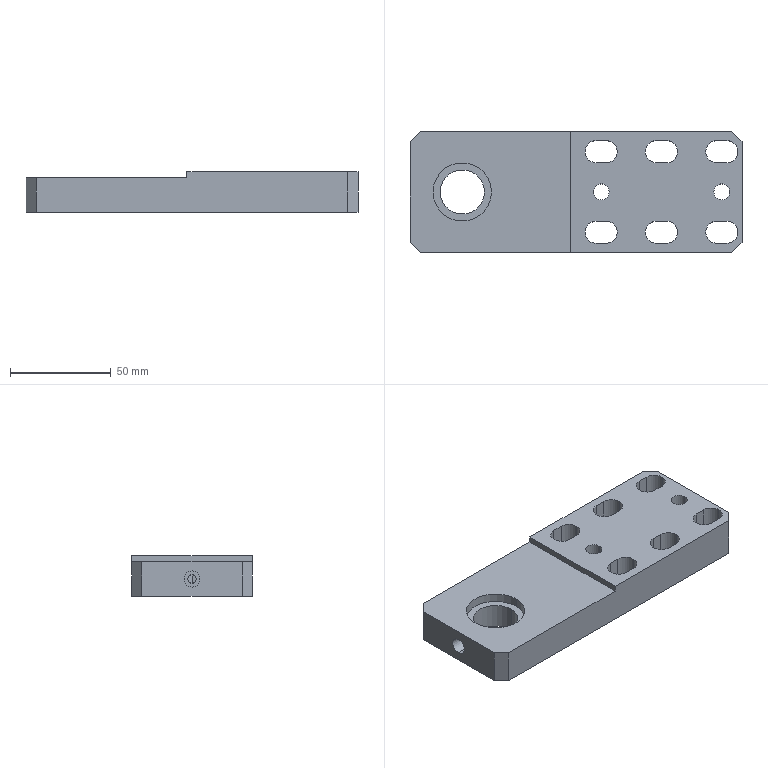Part | STEP file | YCD14007A-08.02.17 Lock Plate | 1 solid | 56 faces | box 165 x 60 x 20 mm | volume 154509 mm3 | cylinder 30 | plane 26 | commonest cylinder face diameters 11 x18 8 x6 4.2 x2 22 x2 29 x2